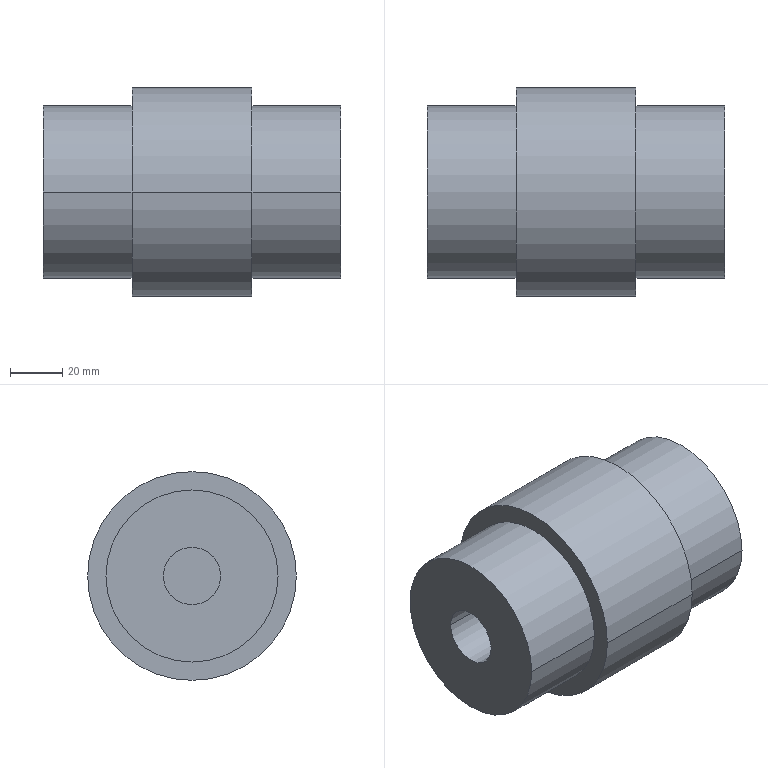Part | SolidWorks | features ICE 2, Revolution 1 | 1 solid | 16 faces | box 114 x 80 x 80 mm | volume 419048 mm3 | cylinder 10 | plane 6 | commonest cylinder face diameters 66 x4 22 x2 28 x2 80 x2
STEP:
#1=CARTESIAN_POINT('',(12.,-21.292,0.));
#2=VERTEX_POINT('',#1);
#3=CARTESIAN_POINT('',(12.,6.708,0.));
#4=VERTEX_POINT('',#3);
#5=CARTESIAN_POINT('',(12.,-7.292,0.));
#6=DIRECTION('',(1.,0.,0.));
#7=DIRECTION('',(0.,1.,0.));
#8=AXIS2_PLACEMENT_3D('',#5,#6,#7);
#9=CIRCLE('',#8,14.);
#10=EDGE_CURVE('',#2,#4,#9,.T.);
#11=ORIENTED_EDGE('',*,*,#10,.F.);
#12=CARTESIAN_POINT('',(57.,-21.292,0.));
#13=VERTEX_POINT('',#12);
#14=CARTESIAN_POINT('',(12.,-21.292,0.));
#15=DIRECTION('',(1.,0.,0.));
#16=VECTOR('',#15,1000.);
#17=LINE('',#14,#16);
#18=EDGE_CURVE('',#2,#13,#17,.T.);
#19=ORIENTED_EDGE('',*,*,#18,.T.);
#20=CARTESIAN_POINT('',(57.,6.708,0.));
#21=VERTEX_POINT('',#20);
#22=CARTESIAN_POINT('',(57.,-7.292,0.));
#23=DIRECTION('',(1.,0.,0.));
#24=DIRECTION('',(0.,1.,0.));
#25=AXIS2_PLACEMENT_3D('',#22,#23,#24);
#26=CIRCLE('',#25,14.);
#27=EDGE_CURVE('',#13,#21,#26,.T.);
#28=ORIENTED_EDGE('',*,*,#27,.T.);
#29=CARTESIAN_POINT('',(12.,6.708,0.));
#30=DIRECTION('',(1.,0.,0.));
#31=VECTOR('',#30,1000.);
#32=LINE('',#29,#31);
#33=EDGE_CURVE('',#4,#21,#32,.T.);
#34=ORIENTED_EDGE('',*,*,#33,.F.);
#35=EDGE_LOOP('',(#11,#19,#28,#34));
#36=FACE_OUTER_BOUND('',#35,.T.);
#37=CARTESIAN_POINT('',(12.,-7.292,0.));
#38=DIRECTION('',(1.,0.,0.));
#39=DIRECTION('',(0.,1.,0.));
#40=AXIS2_PLACEMENT_3D('',#37,#38,#39);
#41=CYLINDRICAL_SURFACE('',#40,14.);
#42=ADVANCED_FACE('',(#36),#41,.F.);
#43=CARTESIAN_POINT('',(-12.,3.708,0.));
#44=VERTEX_POINT('',#43);
#45=CARTESIAN_POINT('',(-12.,-18.292,0.));
#46=VERTEX_POINT('',#45);
#47=CARTESIAN_POINT('',(-12.,-7.292,0.));
#48=DIRECTION('',(-1.,0.,0.));
#49=DIRECTION('',(0.,-1.,0.));
#50=AXIS2_PLACEMENT_3D('',#47,#48,#49);
#51=CIRCLE('',#50,11.);
#52=EDGE_CURVE('',#44,#46,#51,.T.);
#53=ORIENTED_EDGE('',*,*,#52,.F.);
#54=CARTESIAN_POINT('',(-57.,3.708,0.));
#55=VERTEX_POINT('',#54);
#56=CARTESIAN_POINT('',(-12.,3.708,0.));
#57=DIRECTION('',(-1.,0.,0.));
#58=VECTOR('',#57,1000.);
#59=LINE('',#56,#58);
#60=EDGE_CURVE('',#44,#55,#59,.T.);
#61=ORIENTED_EDGE('',*,*,#60,.T.);
#62=CARTESIAN_POINT('',(-57.,-18.292,0.));
#63=VERTEX_POINT('',#62);
#64=CARTESIAN_POINT('',(-57.,-7.292,0.));
#65=DIRECTION('',(-1.,0.,0.));
#66=DIRECTION('',(0.,-1.,0.));
#67=AXIS2_PLACEMENT_3D('',#64,#65,#66);
#68=CIRCLE('',#67,11.);
#69=EDGE_CURVE('',#55,#63,#68,.T.);
#70=ORIENTED_EDGE('',*,*,#69,.T.);
#71=CARTESIAN_POINT('',(-12.,-18.292,0.));
#72=DIRECTION('',(-1.,0.,0.));
#73=VECTOR('',#72,1000.);
#74=LINE('',#71,#73);
#75=EDGE_CURVE('',#46,#63,#74,.T.);
#76=ORIENTED_EDGE('',*,*,#75,.F.);
#77=EDGE_LOOP('',(#53,#61,#70,#76));
#78=FACE_OUTER_BOUND('',#77,.T.);
#79=CARTESIAN_POINT('',(-12.,-7.292,0.));
#80=DIRECTION('',(-1.,0.,0.));
#81=DIRECTION('',(0.,-1.,0.));
#82=AXIS2_PLACEMENT_3D('',#79,#80,#81);
#83=CYLINDRICAL_SURFACE('',#82,11.);
#84=ADVANCED_FACE('',(#78),#83,.F.);
#85=CARTESIAN_POINT('',(57.,-40.292,0.));
#86=VERTEX_POINT('',#85);
#87=CARTESIAN_POINT('',(57.,25.708,0.));
#88=VERTEX_POINT('',#87);
#89=CARTESIAN_POINT('',(57.,-7.292,0.));
#90=DIRECTION('',(-1.,0.,0.));
#91=DIRECTION('',(0.,-1.,0.));
#92=AXIS2_PLACEMENT_3D('',#89,#90,#91);
#93=CIRCLE('',#92,33.);
#94=EDGE_CURVE('',#86,#88,#93,.T.);
#95=ORIENTED_EDGE('',*,*,#94,.T.);
#96=CARTESIAN_POINT('',(23.,25.708,0.));
#97=VERTEX_POINT('',#96);
#98=CARTESIAN_POINT('',(-57.,25.708,0.));
#99=DIRECTION('',(-1.,0.,0.));
#100=VECTOR('',#99,1000.);
#101=LINE('',#98,#100);
#102=EDGE_CURVE('',#88,#97,#101,.T.);
#103=ORIENTED_EDGE('',*,*,#102,.T.);
#104=CARTESIAN_POINT('',(23.,-40.292,0.));
#105=VERTEX_POINT('',#104);
#106=CARTESIAN_POINT('',(23.,-7.292,0.));
#107=DIRECTION('',(-1.,0.,0.));
#108=DIRECTION('',(0.,-1.,0.));
#109=AXIS2_PLACEMENT_3D('',#106,#107,#108);
#110=CIRCLE('',#109,33.);
#111=EDGE_CURVE('',#105,#97,#110,.T.);
#112=ORIENTED_EDGE('',*,*,#111,.F.);
#113=CARTESIAN_POINT('',(-57.,-40.292,0.));
#114=DIRECTION('',(-1.,0.,0.));
#115=VECTOR('',#114,1000.);
#116=LINE('',#113,#115);
#117=EDGE_CURVE('',#86,#105,#116,.T.);
#118=ORIENTED_EDGE('',*,*,#117,.F.);
#119=EDGE_LOOP('',(#95,#103,#112,#118));
#120=FACE_OUTER_BOUND('',#119,.T.);
#121=CARTESIAN_POINT('',(-57.,-7.292,0.));
#122=DIRECTION('',(-1.,0.,0.));
#123=DIRECTION('',(0.,-1.,0.));
#124=AXIS2_PLACEMENT_3D('',#121,#122,#123);
#125=CYLINDRICAL_SURFACE('',#124,33.);
#126=ADVANCED_FACE('',(#120),#125,.T.);
#127=CARTESIAN_POINT('',(23.,-47.292,0.));
#128=VERTEX_POINT('',#127);
#129=CARTESIAN_POINT('',(23.,32.708,0.));
#130=VERTEX_POINT('',#129);
#131=CARTESIAN_POINT('',(23.,-7.292,0.));
#132=DIRECTION('',(-1.,0.,0.));
#133=DIRECTION('',(0.,-1.,0.));
#134=AXIS2_PLACEMENT_3D('',#131,#132,#133);
#135=CIRCLE('',#134,40.);
#136=EDGE_CURVE('',#128,#130,#135,.T.);
#137=ORIENTED_EDGE('',*,*,#136,.T.);
#138=CARTESIAN_POINT('',(-23.,32.708,0.));
#139=VERTEX_POINT('',#138);
#140=CARTESIAN_POINT('',(-57.,32.708,0.));
#141=DIRECTION('',(-1.,0.,0.));
#142=VECTOR('',#141,1000.);
#143=LINE('',#140,#142);
#144=EDGE_CURVE('',#130,#139,#143,.T.);
#145=ORIENTED_EDGE('',*,*,#144,.T.);
#146=CARTESIAN_POINT('',(-23.,-47.292,0.));
#147=VERTEX_POINT('',#146);
#148=CARTESIAN_POINT('',(-23.,-7.292,0.));
#149=DIRECTION('',(-1.,0.,0.));
#150=DIRECTION('',(0.,-1.,0.));
#151=AXIS2_PLACEMENT_3D('',#148,#149,#150);
#152=CIRCLE('',#151,40.);
#153=EDGE_CURVE('',#147,#139,#152,.T.);
#154=ORIENTED_EDGE('',*,*,#153,.F.);
#155=CARTESIAN_POINT('',(-57.,-47.292,0.));
#156=DIRECTION('',(-1.,0.,0.));
#157=VECTOR('',#156,1000.);
#158=LINE('',#155,#157);
#159=EDGE_CURVE('',#128,#147,#158,.T.);
#160=ORIENTED_EDGE('',*,*,#159,.F.);
#161=EDGE_LOOP('',(#137,#145,#154,#160));
#162=FACE_OUTER_BOUND('',#161,.T.);
#163=CARTESIAN_POINT('',(-57.,-7.292,0.));
#164=DIRECTION('',(-1.,0.,0.));
#165=DIRECTION('',(0.,-1.,0.));
#166=AXIS2_PLACEMENT_3D('',#163,#164,#165);
#167=CYLINDRICAL_SURFACE('',#166,40.);
#168=ADVANCED_FACE('',(#162),#167,.T.);
#169=CARTESIAN_POINT('',(-23.,-40.292,0.));
#170=VERTEX_POINT('',#169);
#171=CARTESIAN_POINT('',(-23.,25.708,0.));
#172=VERTEX_POINT('',#171);
#173=CARTESIAN_POINT('',(-23.,-7.292,0.));
#174=DIRECTION('',(-1.,0.,0.));
#175=DIRECTION('',(0.,-1.,0.));
#176=AXIS2_PLACEMENT_3D('',#173,#174,#175);
#177=CIRCLE('',#176,33.);
#178=EDGE_CURVE('',#170,#172,#177,.T.);
#179=ORIENTED_EDGE('',*,*,#178,.T.);
#180=CARTESIAN_POINT('',(-57.,25.708,0.));
#181=VERTEX_POINT('',#180);
#182=CARTESIAN_POINT('',(-57.,25.708,0.));
#183=DIRECTION('',(-1.,0.,0.));
#184=VECTOR('',#183,1000.);
#185=LINE('',#182,#184);
#186=EDGE_CURVE('',#172,#181,#185,.T.);
#187=ORIENTED_EDGE('',*,*,#186,.T.);
#188=CARTESIAN_POINT('',(-57.,-40.292,0.));
#189=VERTEX_POINT('',#188);
#190=CARTESIAN_POINT('',(-57.,-7.292,0.));
#191=DIRECTION('',(-1.,0.,0.));
#192=DIRECTION('',(0.,-1.,0.));
#193=AXIS2_PLACEMENT_3D('',#190,#191,#192);
#194=CIRCLE('',#193,33.);
#195=EDGE_CURVE('',#189,#181,#194,.T.);
#196=ORIENTED_EDGE('',*,*,#195,.F.);
#197=CARTESIAN_POINT('',(-57.,-40.292,0.));
#198=DIRECTION('',(-1.,0.,0.));
#199=VECTOR('',#198,1000.);
#200=LINE('',#197,#199);
#201=EDGE_CURVE('',#170,#189,#200,.T.);
#202=ORIENTED_EDGE('',*,*,#201,.F.);
#203=EDGE_LOOP('',(#179,#187,#196,#202));
#204=FACE_OUTER_BOUND('',#203,.T.);
#205=CARTESIAN_POINT('',(-57.,-7.292,0.));
#206=DIRECTION('',(-1.,0.,0.));
#207=DIRECTION('',(0.,-1.,0.));
#208=AXIS2_PLACEMENT_3D('',#205,#206,#207);
#209=CYLINDRICAL_SURFACE('',#208,33.);
#210=ADVANCED_FACE('',(#204),#209,.T.);
#211=CARTESIAN_POINT('',(-57.,-7.292,0.));
#212=DIRECTION('',(-1.,0.,0.));
#213=DIRECTION('',(0.,-1.,0.));
#214=AXIS2_PLACEMENT_3D('',#211,#212,#213);
#215=CIRCLE('',#214,11.);
#216=EDGE_CURVE('',#63,#55,#215,.T.);
#217=ORIENTED_EDGE('',*,*,#216,.F.);
#218=ORIENTED_EDGE('',*,*,#69,.F.);
#219=EDGE_LOOP('',(#217,#218));
#220=FACE_BOUND('',#219,.T.);
#221=ORIENTED_EDGE('',*,*,#195,.T.);
#222=CARTESIAN_POINT('',(-57.,-7.292,0.));
#223=DIRECTION('',(-1.,0.,0.));
#224=DIRECTION('',(0.,-1.,0.));
#225=AXIS2_PLACEMENT_3D('',#222,#223,#224);
#226=CIRCLE('',#225,33.);
#227=EDGE_CURVE('',#181,#189,#226,.T.);
#228=ORIENTED_EDGE('',*,*,#227,.T.);
#229=EDGE_LOOP('',(#221,#228));
#230=FACE_OUTER_BOUND('',#229,.T.);
#231=CARTESIAN_POINT('',(-57.,-7.292,0.));
#232=DIRECTION('',(1.,0.,0.));
#233=DIRECTION('',(0.,1.,0.));
#234=AXIS2_PLACEMENT_3D('',#231,#232,#233);
#235=PLANE('',#234);
#236=ADVANCED_FACE('',(#220,#230),#235,.F.);
#237=ORIENTED_EDGE('',*,*,#186,.F.);
#238=CARTESIAN_POINT('',(-23.,-7.292,0.));
#239=DIRECTION('',(-1.,0.,0.));
#240=DIRECTION('',(0.,-1.,0.));
#241=AXIS2_PLACEMENT_3D('',#238,#239,#240);
#242=CIRCLE('',#241,33.);
#243=EDGE_CURVE('',#172,#170,#242,.T.);
#244=ORIENTED_EDGE('',*,*,#243,.T.);
#245=ORIENTED_EDGE('',*,*,#201,.T.);
#246=ORIENTED_EDGE('',*,*,#227,.F.);
#247=EDGE_LOOP('',(#237,#244,#245,#246));
#248=FACE_OUTER_BOUND('',#247,.T.);
#249=CARTESIAN_POINT('',(-57.,-7.292,0.));
#250=DIRECTION('',(-1.,0.,0.));
#251=DIRECTION('',(0.,-1.,0.));
#252=AXIS2_PLACEMENT_3D('',#249,#250,#251);
#253=CYLINDRICAL_SURFACE('',#252,33.);
#254=ADVANCED_FACE('',(#248),#253,.T.);
#255=ORIENTED_EDGE('',*,*,#178,.F.);
#256=ORIENTED_EDGE('',*,*,#243,.F.);
#257=EDGE_LOOP('',(#255,#256));
#258=FACE_BOUND('',#257,.T.);
#259=ORIENTED_EDGE('',*,*,#153,.T.);
#260=CARTESIAN_POINT('',(-23.,-7.292,0.));
#261=DIRECTION('',(-1.,0.,0.));
#262=DIRECTION('',(0.,-1.,0.));
#263=AXIS2_PLACEMENT_3D('',#260,#261,#262);
#264=CIRCLE('',#263,40.);
#265=EDGE_CURVE('',#139,#147,#264,.T.);
#266=ORIENTED_EDGE('',*,*,#265,.T.);
#267=EDGE_LOOP('',(#259,#266));
#268=FACE_OUTER_BOUND('',#267,.T.);
#269=CARTESIAN_POINT('',(-23.,25.708,0.));
#270=DIRECTION('',(1.,0.,0.));
#271=DIRECTION('',(0.,1.,0.));
#272=AXIS2_PLACEMENT_3D('',#269,#270,#271);
#273=PLANE('',#272);
#274=ADVANCED_FACE('',(#258,#268),#273,.F.);
#275=ORIENTED_EDGE('',*,*,#144,.F.);
#276=CARTESIAN_POINT('',(23.,-7.292,0.));
#277=DIRECTION('',(-1.,0.,0.));
#278=DIRECTION('',(0.,-1.,0.));
#279=AXIS2_PLACEMENT_3D('',#276,#277,#278);
#280=CIRCLE('',#279,40.);
#281=EDGE_CURVE('',#130,#128,#280,.T.);
#282=ORIENTED_EDGE('',*,*,#281,.T.);
#283=ORIENTED_EDGE('',*,*,#159,.T.);
#284=ORIENTED_EDGE('',*,*,#265,.F.);
#285=EDGE_LOOP('',(#275,#282,#283,#284));
#286=FACE_OUTER_BOUND('',#285,.T.);
#287=CARTESIAN_POINT('',(-57.,-7.292,0.));
#288=DIRECTION('',(-1.,0.,0.));
#289=DIRECTION('',(0.,-1.,0.));
#290=AXIS2_PLACEMENT_3D('',#287,#288,#289);
#291=CYLINDRICAL_SURFACE('',#290,40.);
#292=ADVANCED_FACE('',(#286),#291,.T.);
#293=ORIENTED_EDGE('',*,*,#136,.F.);
#294=ORIENTED_EDGE('',*,*,#281,.F.);
#295=EDGE_LOOP('',(#293,#294));
#296=FACE_OUTER_BOUND('',#295,.T.);
#297=ORIENTED_EDGE('',*,*,#111,.T.);
#298=CARTESIAN_POINT('',(23.,-7.292,0.));
#299=DIRECTION('',(-1.,0.,0.));
#300=DIRECTION('',(0.,-1.,0.));
#301=AXIS2_PLACEMENT_3D('',#298,#299,#300);
#302=CIRCLE('',#301,33.);
#303=EDGE_CURVE('',#97,#105,#302,.T.);
#304=ORIENTED_EDGE('',*,*,#303,.T.);
#305=EDGE_LOOP('',(#297,#304));
#306=FACE_BOUND('',#305,.T.);
#307=CARTESIAN_POINT('',(23.,32.708,0.));
#308=DIRECTION('',(-1.,0.,0.));
#309=DIRECTION('',(0.,-1.,0.));
#310=AXIS2_PLACEMENT_3D('',#307,#308,#309);
#311=PLANE('',#310);
#312=ADVANCED_FACE('',(#296,#306),#311,.F.);
#313=ORIENTED_EDGE('',*,*,#102,.F.);
#314=CARTESIAN_POINT('',(57.,-7.292,0.));
#315=DIRECTION('',(-1.,0.,0.));
#316=DIRECTION('',(0.,-1.,0.));
#317=AXIS2_PLACEMENT_3D('',#314,#315,#316);
#318=CIRCLE('',#317,33.);
#319=EDGE_CURVE('',#88,#86,#318,.T.);
#320=ORIENTED_EDGE('',*,*,#319,.T.);
#321=ORIENTED_EDGE('',*,*,#117,.T.);
#322=ORIENTED_EDGE('',*,*,#303,.F.);
#323=EDGE_LOOP('',(#313,#320,#321,#322));
#324=FACE_OUTER_BOUND('',#323,.T.);
#325=CARTESIAN_POINT('',(-57.,-7.292,0.));
#326=DIRECTION('',(-1.,0.,0.));
#327=DIRECTION('',(0.,-1.,0.));
#328=AXIS2_PLACEMENT_3D('',#325,#326,#327);
#329=CYLINDRICAL_SURFACE('',#328,33.);
#330=ADVANCED_FACE('',(#324),#329,.T.);
#331=CARTESIAN_POINT('',(57.,-7.292,0.));
#332=DIRECTION('',(1.,0.,0.));
#333=DIRECTION('',(0.,1.,0.));
#334=AXIS2_PLACEMENT_3D('',#331,#332,#333);
#335=CIRCLE('',#334,14.);
#336=EDGE_CURVE('',#21,#13,#335,.T.);
#337=ORIENTED_EDGE('',*,*,#336,.F.);
#338=ORIENTED_EDGE('',*,*,#27,.F.);
#339=EDGE_LOOP('',(#337,#338));
#340=FACE_BOUND('',#339,.T.);
#341=ORIENTED_EDGE('',*,*,#94,.F.);
#342=ORIENTED_EDGE('',*,*,#319,.F.);
#343=EDGE_LOOP('',(#341,#342));
#344=FACE_OUTER_BOUND('',#343,.T.);
#345=CARTESIAN_POINT('',(57.,25.708,0.));
#346=DIRECTION('',(-1.,0.,0.));
#347=DIRECTION('',(0.,-1.,0.));
#348=AXIS2_PLACEMENT_3D('',#345,#346,#347);
#349=PLANE('',#348);
#350=ADVANCED_FACE('',(#340,#344),#349,.F.);
#351=ORIENTED_EDGE('',*,*,#60,.F.);
#352=CARTESIAN_POINT('',(-12.,-7.292,0.));
#353=DIRECTION('',(-1.,0.,0.));
#354=DIRECTION('',(0.,-1.,0.));
#355=AXIS2_PLACEMENT_3D('',#352,#353,#354);
#356=CIRCLE('',#355,11.);
#357=EDGE_CURVE('',#46,#44,#356,.T.);
#358=ORIENTED_EDGE('',*,*,#357,.F.);
#359=ORIENTED_EDGE('',*,*,#75,.T.);
#360=ORIENTED_EDGE('',*,*,#216,.T.);
#361=EDGE_LOOP('',(#351,#358,#359,#360));
#362=FACE_OUTER_BOUND('',#361,.T.);
#363=CARTESIAN_POINT('',(-12.,-7.292,0.));
#364=DIRECTION('',(-1.,0.,0.));
#365=DIRECTION('',(0.,-1.,0.));
#366=AXIS2_PLACEMENT_3D('',#363,#364,#365);
#367=CYLINDRICAL_SURFACE('',#366,11.);
#368=ADVANCED_FACE('',(#362),#367,.F.);
#369=ORIENTED_EDGE('',*,*,#357,.T.);
#370=ORIENTED_EDGE('',*,*,#52,.T.);
#371=EDGE_LOOP('',(#369,#370));
#372=FACE_OUTER_BOUND('',#371,.T.);
#373=CARTESIAN_POINT('',(-12.,-7.292,0.));
#374=DIRECTION('',(-1.,0.,0.));
#375=DIRECTION('',(0.,-1.,0.));
#376=AXIS2_PLACEMENT_3D('',#373,#374,#375);
#377=PLANE('',#376);
#378=ADVANCED_FACE('',(#372),#377,.T.);
#379=ORIENTED_EDGE('',*,*,#18,.F.);
#380=CARTESIAN_POINT('',(12.,-7.292,0.));
#381=DIRECTION('',(1.,0.,0.));
#382=DIRECTION('',(0.,1.,0.));
#383=AXIS2_PLACEMENT_3D('',#380,#381,#382);
#384=CIRCLE('',#383,14.);
#385=EDGE_CURVE('',#4,#2,#384,.T.);
#386=ORIENTED_EDGE('',*,*,#385,.F.);
#387=ORIENTED_EDGE('',*,*,#33,.T.);
#388=ORIENTED_EDGE('',*,*,#336,.T.);
#389=EDGE_LOOP('',(#379,#386,#387,#388));
#390=FACE_OUTER_BOUND('',#389,.T.);
#391=CARTESIAN_POINT('',(12.,-7.292,0.));
#392=DIRECTION('',(1.,0.,0.));
#393=DIRECTION('',(0.,1.,0.));
#394=AXIS2_PLACEMENT_3D('',#391,#392,#393);
#395=CYLINDRICAL_SURFACE('',#394,14.);
#396=ADVANCED_FACE('',(#390),#395,.F.);
#397=ORIENTED_EDGE('',*,*,#385,.T.);
#398=ORIENTED_EDGE('',*,*,#10,.T.);
#399=EDGE_LOOP('',(#397,#398));
#400=FACE_OUTER_BOUND('',#399,.T.);
#401=CARTESIAN_POINT('',(12.,-7.292,0.));
#402=DIRECTION('',(1.,0.,0.));
#403=DIRECTION('',(0.,1.,0.));
#404=AXIS2_PLACEMENT_3D('',#401,#402,#403);
#405=PLANE('',#404);
#406=ADVANCED_FACE('',(#400),#405,.T.);
#407=CLOSED_SHELL('',(#42,#84,#126,#168,#210,#236,#254,#274,#292,#312,#330,#350,#368,#378,#396,#406));
#408=MANIFOLD_SOLID_BREP('',#407);
#409=CARTESIAN_POINT('',(0.,0.,0.));
#410=DIRECTION('',(0.,0.,1.));
#411=DIRECTION('',(1.,0.,0.));
#412=AXIS2_PLACEMENT_3D('',#409,#410,#411);
#413=(LENGTH_UNIT()NAMED_UNIT(*)SI_UNIT(.MILLI.,.METRE.));
#414=UNCERTAINTY_MEASURE_WITH_UNIT(LENGTH_MEASURE(0.00001),#413,'','');
#415=(NAMED_UNIT(*)PLANE_ANGLE_UNIT()SI_UNIT($,.RADIAN.));
#416=(NAMED_UNIT(*)SI_UNIT($,.STERADIAN.)SOLID_ANGLE_UNIT());
#417=(GEOMETRIC_REPRESENTATION_CONTEXT(3)GLOBAL_UNCERTAINTY_ASSIGNED_CONTEXT((#414))GLOBAL_UNIT_ASSIGNED_CONTEXT((#413,#415,#416))REPRESENTATION_CONTEXT('',''));
#418=ADVANCED_BREP_SHAPE_REPRESENTATION('',(#408,#412),#417);